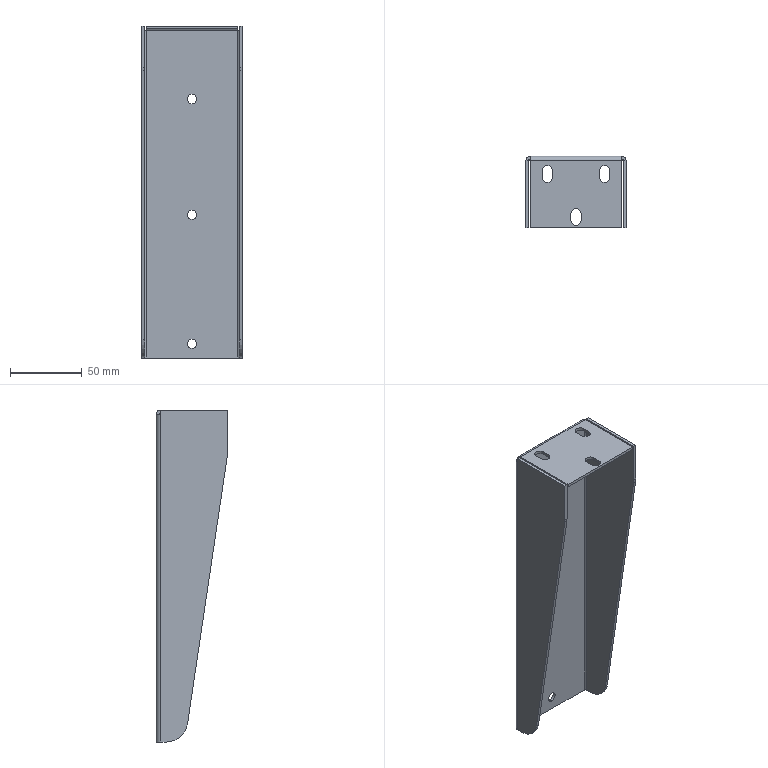Part | SolidWorks | features ICE 3, EdgeFlange 1, Fillet 1, FlatPattern 1, SMBaseFlange 1, SheetMetal 1 | 1 solid | 56 faces | box 70 x 50 x 232 mm | volume 69334 mm3 | plane 34 | cylinder 22 | commonest cylinder face diameters 6.4 x6 7 x6 30 x4 2 x3 6 x3